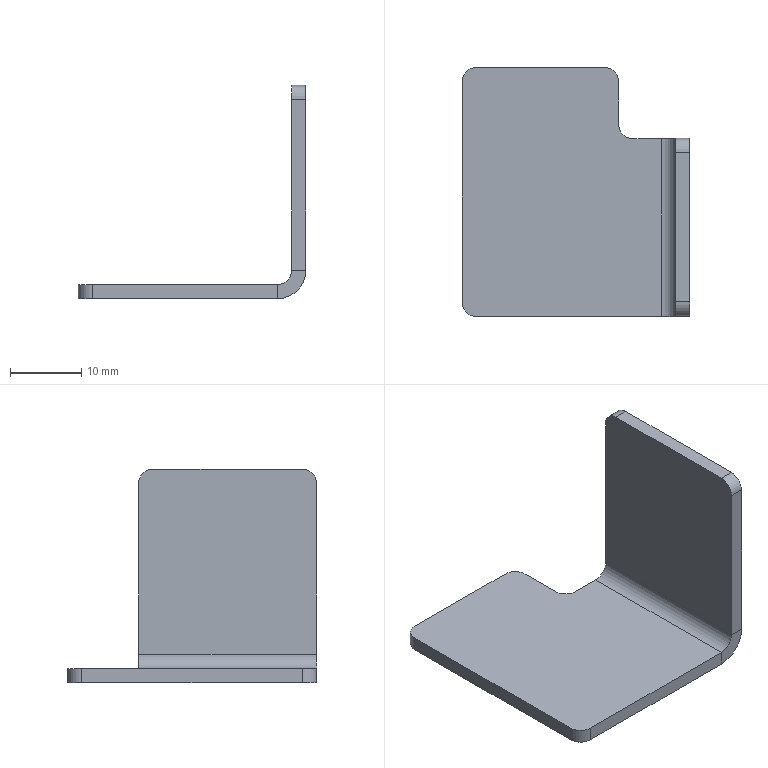Part | STEP file | 001-011-Blanking flip end sensor mounting seat | 1 solid | 22 faces | box 32 x 35 x 30 mm | volume 3369 mm3 | plane 14 | cylinder 8 | commonest cylinder face diameters 4 x7 8 x1